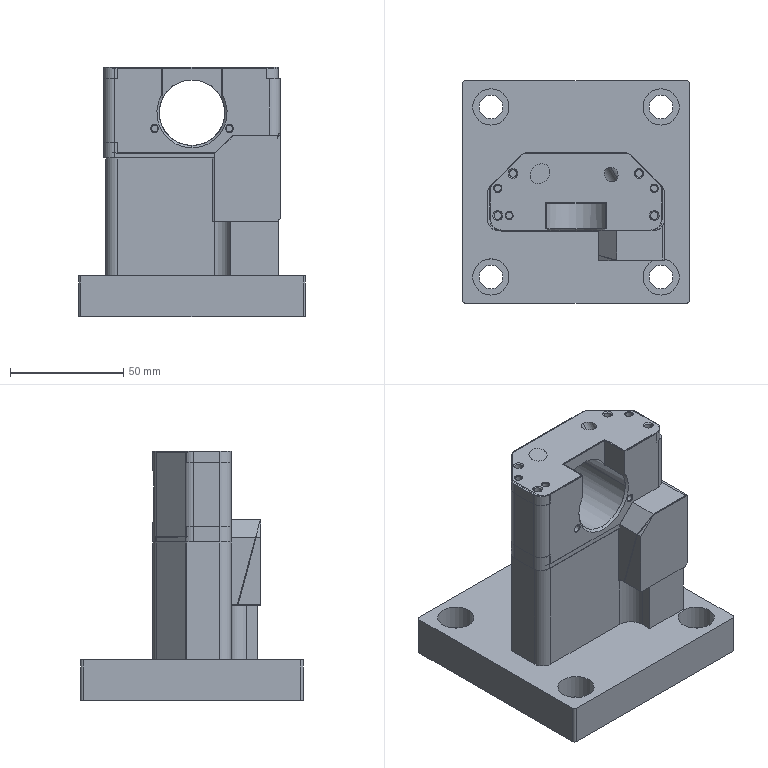NC program | NX | posted with a generic post | part box 100 x 98 x 110 mm
Lines 1 to 816 of 6635:
N10 G17 G21 G94 G90
(ADAPTIVE_MILLING_1 , TOOL : D16-48-D16-100-3T-ROUGH)
N12 T02 M6
N14 G54
N16 G17 G0 G90 X-56.885 Y-40.205 B0. C0. S6500 M3
N18 G43 Z71. H2
N20 Z43.15
N22 G94 G1 X-56.737 Y-40.182 Z42.213 F3000.
N24 X-56.588 Y-40.16 Z41.842
N26 X-56.44 Y-40.138 Z41.57
N28 X-56.291 Y-40.116 Z41.35
N30 X-56.143 Y-40.093 Z41.166
N32 X-55.995 Y-40.071 Z41.008
N34 X-55.846 Y-40.049 Z40.87
N36 X-55.698 Y-40.027 Z40.75
N38 X-55.55 Y-40.004 Z40.645
N40 X-55.401 Y-39.982 Z40.552
N42 X-55.253 Y-39.96 Z40.471
N44 X-55.105 Y-39.937 Z40.4
N46 X-54.956 Y-39.915 Z40.34
N48 X-54.808 Y-39.893 Z40.288
N50 X-54.66 Y-39.871 Z40.245
N52 X-54.511 Y-39.848 Z40.211
N54 X-54.363 Y-39.826 Z40.184
N56 X-54.215 Y-39.804 Z40.165
N58 X-54.066 Y-39.782 Z40.154
N60 X-53.918 Y-39.759 Z40.15
N62 X-51.733 Y-39.431
N64 G3 X-50.362 Y-37.706 R1.616
N66 G2 X-50.32 Y-34.589 R11.935
N68 G3 X-50.025 Y-25.185 R132.104
N70 G1 X-50. Y-12.98
N72 X-49.999 Y17.769
N74 G2 X-47.614 Y23.395 R8.513
N76 X-42.154 Y26.798 R13.179
N78 X-35.417 Y28.08 R28.008
N80 X-26.55 Y28.398 R123.992
N82 G1 X-12.675 Y28.431
N84 X39.401 Y28.429
N86 G2 X45.01 Y26.001 R8.56
N88 X48.428 Y20.406 R13.296
N90 X49.673 Y13.535 R29.032
N92 X49.978 Y3.542 R145.98
N94 G1 X50. Y-8.708
N96 X49.999 Y-30.87
N98 G2 X47.636 Y-36.505 R8.508
N100 X42.184 Y-39.92 R13.098
N102 X35.323 Y-41.215 R28.218
N104 X24.956 Y-41.538 R142.942
N106 G1 X12.831 Y-41.56
N108 X-38.711 Y-41.565
N110 G2 X-43.908 Y-39.391 R8.253
N112 X-47.391 Y-33.973 R12.678
N114 X-48.662 Y-27.362 R26.87
N116 X-48.98 Y-17.119 R138.758
N118 G1 X-49. Y-5.369
N120 X-48.995 Y14.156
N122 G2 X-44.813 Y22.643 R11.417
N124 X-38.379 Y25.922 R17.037
N126 X-30.735 Y27.117 R37.582
N128 X-19.116 Y27.415 R192.657
N130 G1 X-8.366 Y27.431
N132 X35.711 Y27.427
N134 G2 X44.199 Y23.258 R11.416
N136 X47.512 Y16.729 R17.072
N138 X48.682 Y9.208 R37.658
N140 X48.981 Y-2.036 R184.867
N142 G1 X48.999 Y-12.661
N144 X48.995 Y-27.28
N146 G2 X44.631 Y-35.925 R11.455
N148 X38.055 Y-39.14 R17.391
N150 X30.4 Y-40.267 R39.59
N152 X18.155 Y-40.547 R216.039
N154 G1 X8.905 Y-40.56
N156 X-34.711 Y-40.566
N158 G2 X-43.314 Y-36.39 R11.266
N160 X-46.587 Y-29.818 R17.057
N162 X-47.7 Y-22.413 R38.181
N164 X-47.987 Y-10.418 R203.457
N166 G1 X-47.999 Y-0.793
N168 G2 X-47.978 Y11.392 R882.053
N170 X-42.319 Y21.918 R13.288
N172 X-35.382 Y25.006 R19.979
N174 X-26.971 Y26.15 R45.911
N176 X-13.975 Y26.42 R250.02
N178 G1 X-4.35 Y26.43
N180 X32.086 Y26.429
N182 G2 X38.948 Y24.812 R13.899
N184 X44.742 Y18.723 R14.548
N186 X47.104 Y11.243 R24.627
N188 X47.861 Y2.156 R69.648
N190 X47.997 Y-13.218 R577.956
N192 X47.972 Y-24.654 R605.431
N194 X42.312 Y-35.05 R13.267
N196 X35.139 Y-38.192 R20.2
N198 X26.721 Y-39.291 R47.551
N200 X12.475 Y-39.553 R284.691
N202 G1 X4.225 Y-39.56
N204 X-31.335 Y-39.564
N206 G2 X-38.711 Y-37.564 R13.487
N208 X-44.102 Y-31.274 R14.868
N210 X-46.22 Y-23.842 R26.112
N212 X-46.894 Y-14.372 R79.249
N214 X-46.999 Y3.002 R851.623
N216 X-46.939 Y9.401 R131.04
N218 X-40.169 Y21.069 R14.609
N220 X-32.657 Y24.096 R22.601
N222 X-23.607 Y25.181 R54.343
N224 X-8.485 Y25.425 R334.897
N226 G1 X-1.61 Y25.43
N228 X28.915 Y25.429
N230 G2 X34.482 Y24.776 R19.528
N232 X42.634 Y18.602 R14.637
N234 X45.663 Y11.091 R22.586
N236 X46.742 Y2.166 R53.819
N238 X46.993 Y-13.081 R329.877
N240 X46.964 Y-22.08 R344.498
N242 X44.364 Y-30.176 R14.873
N244 X37.58 Y-35.614 R16.432
N246 X29.765 Y-37.748 R28.844
N248 X19.921 Y-38.444 R85.653
N250 X1.046 Y-38.56 R885.601
N252 G1 X-28.085 Y-38.564
N254 G2 X-33.65 Y-37.896 R19.153
N256 X-41.719 Y-31.705 R14.562
N258 X-44.704 Y-24.187 R22.662
N260 X-45.755 Y-15.259 R54.73
N262 X-45.992 Y-1.012 R322.025
N264 X-45.945 Y6.862 R209.476
N266 X-43.914 Y14.394 R16.668
N268 X-37.081 Y20.814 R16.454
N270 X-29.017 Y23.388 R27.307
N272 X-19.313 Y24.256 R73.092
N274 X-2.314 Y24.428 R541.419
N276 G1 X25.961 Y24.429
N278 G2 X31.558 Y23.989 R26.965
N280 X41.465 Y17.077 R15.491
N282 X44.553 Y9.453 R23.605
N284 X45.709 Y0.287 R54.619
N286 X45.989 Y-14.334 R295.948
N288 X45.906 Y-20.582 R95.145
N290 X42.831 Y-29.171 R15.836
N292 X35.625 Y-34.633 R17.635
N294 X27.542 Y-36.743 R31.272
N296 X17.446 Y-37.439 R91.485
N298 X-1.803 Y-37.56 R888.945
N300 G1 X-25.46 Y-37.562
N302 G2 X-31.169 Y-37.01 R23.929
N304 X-40.551 Y-30.162 R15.425
N306 X-43.62 Y-22.412 R23.796
N308 X-44.734 Y-13.114 R56.809
N310 X-44.951 Y4.382 R306.489
N312 X-43.611 Y11.214 R19.554
N314 X-36.477 Y19.2 R16.579
N316 X-28.528 Y22.101 R26.152
N318 X-18.847 Y23.178 R63.148
N320 X-2.725 Y23.424 R380.785
N322 G1 X4.15 Y23.429
N324 X23.8 Y23.427
N326 G2 X29.771 Y22.955 R29.934
N328 X40.427 Y15.466 R16.289
N330 X43.558 Y7.471 R25.044
N332 X44.72 Y-2.198 R59.034
N334 X44.947 Y-17.444 R256.134
N336 X43.633 Y-24.281 R19.663
N338 X36.608 Y-32.247 R16.569
N340 X28.551 Y-35.222 R25.928
N342 X18.746 Y-36.31 R63.537
N344 X2.624 Y-36.554 R385.545
N346 G1 X-4.251 Y-36.56
N348 X-22.96 Y-36.561
N350 G2 X-28.93 Y-36.077 R29.329
N352 X-39.456 Y-28.627 R16.21
N354 X-42.552 Y-20.738 R24.98
N356 X-43.714 Y-11.194 R58.416
N358 X-43.921 Y2.676 R191.786
N360 X-42.612 Y9.519 R20.813
N362 X-35.365 Y17.907 R17.11
N364 X-27.077 Y21.017 R26.557
N366 X-17.027 Y22.162 R64.138
N368 X-1.406 Y22.421 R359.586
N370 G1 X6.844 Y22.428
N372 X21.336 Y22.427
N374 G2 X27.565 Y22.023 R36.993
N376 X39.255 Y14.153 R16.957
N378 X42.44 Y6.164 R25.668
N380 X43.675 Y-3.497 R58.226
N382 X43.904 Y-15.867 R156.374
N384 X42.486 Y-22.938 R20.39
N386 X35.181 Y-31.143 R17.173
N388 X26.868 Y-34.186 R27.044
N390 X16.815 Y-35.3 R65.737
N392 X0.318 Y-35.554 R391.668
N394 G1 X-6.557 Y-35.559
N396 X-20.085 Y-35.561
N398 G2 X-26.319 Y-35.213 R40.275
N400 X-38.402 Y-27.115 R16.941
N402 X-41.53 Y-18.984 R26.096
N404 X-42.713 Y-9.066 R61.493
N406 X-42.876 Y1.055 R124.215
N408 X-41.416 Y8.372 R21.436
N410 X-34.005 Y16.803 R17.662
N412 X-25.863 Y19.901 R27.04
N414 X-15.948 Y21.114 R62.015
N416 X-0.077 Y21.418 R322.023
N418 G1 X9.548 Y21.427
N420 G2 X21.697 Y21.388 R659.225
N422 X28.477 Y20.39 R25.036
N424 X38.259 Y12.625 R17.561
N426 X41.476 Y4.261 R26.907
N428 X42.691 Y-5.78 R62.743
N430 X42.826 Y-14.65 R92.117
N432 X41.063 Y-22.274 R20.204
N434 X33.684 Y-30.116 R17.819
N436 X25.377 Y-33.131 R27.885
N438 X15.326 Y-34.275 R66.109
N440 X-0.42 Y-34.55 R353.217
N442 G1 X-8.67 Y-34.559
N444 G2 X-20.835 Y-34.52 R627.473
N446 X-27.492 Y-33.541 R24.81
N448 X-37.297 Y-25.753 R17.501
N450 X-40.496 Y-17.386 R26.951
N452 X-41.703 Y-7.219 R63.63
N454 X-41.73 Y0.776 R63.896
N456 X-39.361 Y8.998 R19.551
N458 X-31.841 Y16.186 R18.657
N460 X-23.353 Y19.073 R29.671
N462 X-12.92 Y20.17 R72.683
N464 X4.327 Y20.422 R423.71
N466 G1 X11.202 Y20.427
N468 G2 X20.585 Y20.356 R267.632
N470 X27.702 Y19.122 R24.347
N472 X37.307 Y11.071 R18.155
N474 X40.485 Y2.552 R28.12
N476 X41.708 Y-8.117 R66.144
N478 X41.556 Y-15.231 R42.135
N480 X32.931 Y-28.678 R17.947
N482 X24.577 Y-31.94 R27.303
N484 X14.667 Y-33.207 R61.606
N486 X-0.578 Y-33.544 R290.453
N488 G1 X-11.578 Y-33.559
N490 G2 X-20.209 Y-33.463 R178.586
N492 X-27.523 Y-31.969 R22.618
N494 X-36.369 Y-24.155 R18.163
N496 X-39.489 Y-15.738 R28.141
N498 X-40.666 Y-1.194 R61.873
N500 X-38.682 Y6.89 R20.653
N502 X-30.912 Y14.894 R18.781
N504 X-22.467 Y17.924 R29.31
N506 X-11.921 Y19.13 R69.186
N508 X4.325 Y19.417 R361.409
N510 X18.2 Y19.377 R613.553
N512 X25.241 Y18.419 R28.599
N514 X36.144 Y9.914 R18.54
N516 X39.381 Y1.424 R28.401
N518 X40.594 Y-11.988 R55.222
N520 X38.515 Y-20.291 R20.184
N522 X30.766 Y-28.096 R18.808
N524 X22.189 Y-31.105 R29.746
N526 X11.763 Y-32.266 R70.65
N528 X-5.234 Y-32.551 R382.948
N530 X-17.483 Y-32.504 R470.412
N532 X-24.396 Y-31.527 R27.9
N534 X-35.1 Y-23.172 R18.455
N536 X-38.338 Y-14.811 R27.977
N538 X-39.5 Y-2.275 R48.395
N540 X-37.123 Y6.453 R20.027
N542 X-29.457 Y13.912 R19.217
N544 X-20.637 Y16.977 R30.448
N546 X-9.835 Y18.145 R73.801
N548 X7.662 Y18.42 R411.362
N550 X17.535 Y18.332 R229.778
N552 X24.782 Y17.099 R26.546
N554 X35.03 Y8.718 R18.923
N556 X38.384 Y-0.143 R29.074
N558 X39.392 Y-11.067 R43.089
N560 X36.714 Y-20.213 R19.386
N562 X28.974 Y-27.287 R19.454
N564 X20.203 Y-30.184 R31.503
N566 X9.393 Y-31.294 R77.133
N568 X-7.729 Y-31.552 R429.437
N570 X-16.602 Y-31.465 R200.678
N572 X-23.848 Y-30.23 R26.387
N574 X-34.069 Y-21.832 R18.881
N576 X-37.371 Y-13.1 R28.888
N578 X-38.256 Y-2.92 R37.59
N580 X-34.78 Y7.115 R19.055
N582 X-26.856 Y13.521 R20.464
N584 X-17.776 Y16.217 R34.328
N586 X-6.452 Y17.215 R89.134
N588 X14.92 Y17.367 R468.732
N590 X22.219 Y16.435 R31.978
N592 X33.937 Y7.516 R19.297
N594 X37.361 Y-1.577 R29.292
N596 X38.091 Y-10.767 R32.807
N598 X29.508 Y-25.154 R18.422
N600 X20.969 Y-28.686 R27.691
N602 X10.583 Y-30.136 R60.771
N604 X-4.535 Y-30.534 R261.029
N606 X-15.034 Y-30.457 R229.195
N608 X-22.409 Y-29.229 R27.63
N610 X-33.052 Y-20.497 R19.274
N612 X-36.486 Y-10.886 R29.362
N614 X-36.799 Y-2.179 R27.378
N616 X-28.604 Y10.743 R18.461
N618 X-20.027 Y14.431 R27.428
N620 X-9.778 Y15.952 R58.414
N622 X4.088 Y16.388 R225.599
N624 X14.461 Y16.315 R208.549
N626 X21.964 Y15.091 R28.827
N628 X32.87 Y6.301 R19.628
N630 X36.627 Y-5.021 R29.285
N632 X36.056 Y-13.816 R21.747
N634 X28.557 Y-23.866 R18.306
N636 X19.97 Y-27.564 R27.369
N638 X9.721 Y-29.083 R58.654
N640 X-5.395 Y-29.528 R242.488
N642 X-14.517 Y-29.388 R129.556
N644 X-22.198 Y-27.8 R25.596
N646 X-31.983 Y-19.279 R19.641
N648 X-35.62 Y-5.029 R27.098
N650 X-27.736 Y9.396 R18.221
N652 X-19.469 Y13.192 R26.585
N654 X-9.247 Y14.871 R54.684
N656 X5.241 Y15.381 R206.257
N658 X14.362 Y15.218 R113.494
N660 X22.148 Y13.529 R25.672
N662 X31.918 Y4.911 R19.991
N664 X35.4 Y-8.094 R25.444
N666 X27.944 Y-22.318 R17.842
N668 X19.493 Y-26.297 R26.146
N670 X9.399 Y-27.984 R53.896
N672 X-4.963 Y-28.509 R200.139
N674 X-13.708 Y-28.326 R99.733
N676 X-21.592 Y-26.492 R24.816
N678 X-31.116 Y-17.723 R19.984
N680 X-34.164 Y-5.853 R23.484
N682 X-27.199 Y7.764 R17.675
N684 X-18.927 Y11.928 R25.352
N686 X-9.107 Y13.746 R50.121
N688 X5.126 Y14.358 R171.985
N690 X13.744 Y14.135 R85.535
N692 X21.938 Y12.044 R24.427
N694 X31.299 Y2.906 R20.376
N696 X33.883 Y-7.671 R21.757
N698 X27.536 Y-20.534 R17.229
N700 X19.275 Y-24.924 R24.472
N702 X9.353 Y-26.845 R48.428
N704 X-4.504 Y-27.48 R161.733
N706 X-13.12 Y-27.231 R78.292
N708 X-21.395 Y-24.972 R23.686
N710 X-30.848 Y-14.861 R20.337
N712 X-32.463 Y-4.616 R19.331
N714 X-26.283 Y6.366 R17.162
N716 X-18.15 Y10.718 R24.431
N718 X-8.356 Y12.668 R47.689
N720 X10.372 Y13.252 R148.984
N722 X18.127 Y12.014 R30.686
N724 X32.213 Y-5.312 R20.183
N726 X26.806 Y-18.907 R16.489
N728 X18.883 Y-23.56 R23.107
N730 X9.386 Y-25.672 R43.694
N732 X-4.461 Y-26.442 R132.029
N734 X-12.822 Y-26.083 R60.203
N736 X-21.752 Y-23.06 R22.292
N738 X-30.735 Y-9.76 R19.35
N740 X-26.025 Y4.269 R16.135
N742 X-18.119 Y9.214 R22.417
N744 X-8.775 Y11.44 R41.528
N746 X9.565 Y12.189 R116.003
N748 X17.42 Y10.809 R29.248
N750 X29.52 Y-0.727 R19.418
N752 X26.199 Y-17.008 R15.583
N754 X18.558 Y-22.115 R21.467
N756 X9.256 Y-24.489 R39.196
N758 X-4.831 Y-25.39 R108.385
N760 X-12.926 Y-24.835 R45.533
N762 X-22.552 Y-20.614 R20.979
N764 X-28.744 Y-10.981 R17.552
N766 X-25.355 Y2.321 R15.122
N768 X-17.975 Y7.658 R20.555
N770 X-8.847 Y10.21 R36.601
N772 X8.728 Y11.112 R92.536
N774 X16.917 Y9.517 R27.854
N776 X26.436 Y1.819 R18.73
N778 X25.351 Y-15.128 R14.581
N780 X18.133 Y-20.63 R19.791
N782 X9.532 Y-23.203 R34.399
N784 X-4.284 Y-24.311 R85.783
N786 X-12.491 Y-23.634 R39.783
N788 X-21.782 Y-19.202 R20.242
N790 X-26.884 Y-10.793 R15.424
N792 X-24.071 Y0.859 R14.209
N794 X-16.905 Y6.435 R19.497
N796 X-8.072 Y9.086 R34.247
N798 X7.995 Y10.011 R74.707
N800 X16.274 Y8.255 R26.491
N802 X24.04 Y2.318 R17.591
N804 X24.294 Y-13.173 R13.493
N806 X17.705 Y-19.032 R18.06
N808 X9.342 Y-21.94 R30.46
N810 X-7.325 Y-23.097 R67.662
N812 X-15.467 Y-21.303 R25.558
N814 X-22.541 Y-15.899 R16.613
N816 X-23.18 Y-1.523 R12.975
N818 X-16.814 Y4.611 R17.312
N820 X-8.397 Y7.715 R29.048
N822 X7.388 Y8.877 R59.899
N824 X15.627 Y6.964 R24.802
N826 X22.062 Y1.935 R15.623
N828 X22.92 Y-11.206 R12.412
N830 X16.932 Y-17.464 R16.395
N832 X8.812 Y-20.694 R27.127
N834 X-6.835 Y-21.94 R54.242
N836 X-14.807 Y-19.989 R23.437
N838 X-20.733 Y-15.113 R14.174
N840 X-21.437 Y-3.087 R11.966
N842 X-15.55 Y3.276 R15.99
N844 X-7.591 Y6.512 R26.353
N846 X7.179 Y7.676 R47.817
N848 X14.763 Y5.715 R22.244
N850 X20.403 Y0.735 R12.949
N852 X20.865 Y-9.951 R11.505
N854 X15.319 Y-16.264 R15.291
N856 X7.523 Y-19.575 R25.019
N858 X-6.616 Y-20.717 R43.089
N860 X-13.591 Y-18.856 R20.486
N862 X-19.066 Y-13.559 R11.694
N864 X-19.035 Y-3.884 R11.205
N866 X-13.507 Y2.293 R15.092
N868 X-5.798 Y5.496 R24.694
N870 X6.984 Y6.417 R37.765
N872 X13.441 Y4.573 R18.418
N874 X19.141 Y-3.484 R10.505
N876 X16.905 Y-11.621 R11.616
N878 X10.678 Y-16.716 R16.592
N880 X1.833 Y-19.288 R28.96
N882 X-7.381 Y-19.276 R30.623
N884 X-12.847 Y-17.238 R14.001
N886 X-16.944 Y-6.618 R9.897
N888 X-12.787 Y0.066 R12.881
N890 X-5.683 Y3.922 R19.713
N892 X6.667 Y5.083 R29.045
N894 X11.824 Y3.303 R12.563
N896 X15.928 Y-6.115 R9.363
N898 X12.061 Y-13.089 R12.147
N900 X5.016 Y-17.036 R18.525
N902 X-5.477 Y-18.093 R24.979
N904 X-10.71 Y-15.913 R9.896
N906 X-13.65 Y-7.689 R8.937
N908 X-9.995 Y-0.995 R11.714
N910 X-2.938 Y2.916 R17.429
N912 X4.721 Y3.748 R20.39
N914 X12.159 Y-4.269 R8.111
N916 X9.554 Y-11.257 R10.475
N918 X2.679 Y-15.715 R15.051
N920 X-2.23 Y-16.538 R14.881
N922 X-8.827 Y-11.184 R7.024
N924 X-7.719 Y-4.212 R9.092
N926 X-1.402 Y0.889 R12.075
N928 X2.442 Y0.365 R4.734
N930 X6.261 Y-5.107 R8.144
N932 G1 X6.388 Y-5.846
N934 X6.409 Y-5.994 Z40.154
N936 X6.43 Y-6.143 Z40.165
N938 X6.451 Y-6.291 Z40.184
N940 X6.472 Y-6.44 Z40.211
N942 X6.492 Y-6.588 Z40.245
N944 X6.513 Y-6.737 Z40.288
N946 X6.534 Y-6.886 Z40.34
N948 X6.555 Y-7.034 Z40.4
N950 X6.576 Y-7.183 Z40.471
N952 X6.596 Y-7.331 Z40.552
N954 X6.617 Y-7.48 Z40.645
N956 X6.638 Y-7.628 Z40.75
N958 X6.659 Y-7.777 Z40.87
N960 X6.68 Y-7.925 Z41.008
N962 X6.701 Y-8.074 Z41.166
N964 X6.721 Y-8.222 Z41.35
N966 X6.742 Y-8.371 Z41.57
N968 X6.763 Y-8.52 Z41.842
N970 X6.784 Y-8.668 Z42.213
N972 X6.805 Y-8.817 Z43.15
N974 G0 Z71.
(ADAPTIVE_MILLING_1_COPY , TOOL : D16-48-D16-100-3T-ROUGH)
N976 X-58.104 Y-13.402
N978 Z3.
N980 G1 X-57.954 Y-13.401 Z2.063
N982 X-57.804 Y-13.399 Z1.692
N984 X-57.654 Y-13.398 Z1.42
N986 X-57.504 Y-13.396 Z1.2
N988 X-57.354 Y-13.395 Z1.016
N990 X-57.204 Y-13.393 Z0.858
N992 X-57.054 Y-13.391 Z0.72
N994 X-56.904 Y-13.39 Z0.6
N996 X-56.754 Y-13.388 Z0.495
N998 X-56.604 Y-13.387 Z0.402
N1000 X-56.454 Y-13.385 Z0.321
N1002 X-56.304 Y-13.384 Z0.25
N1004 X-56.154 Y-13.382 Z0.19
N1006 X-56.004 Y-13.38 Z0.138
N1008 X-55.854 Y-13.379 Z0.095
N1010 X-55.704 Y-13.377 Z0.061
N1012 X-55.554 Y-13.376 Z0.034
N1014 X-55.404 Y-13.374 Z0.015
N1016 X-55.254 Y-13.373 Z0.004
N1018 X-55.104 Y-13.371 Z0.
N1020 X-52.595 Y-13.345
N1022 G3 X-51.099 Y-12.298 R1.616
N1024 X-50.374 Y-8.84 R12.888
N1026 X-50.039 Y-0.285 R101.881
N1028 G1 X-50.001 Y11.645
N1030 G2 X-49.977 Y18.269 R246.209
N1032 X-47.177 Y23.842 R8.816
N1034 X-41.44 Y27.029 R13.966
N1036 X-34.42 Y28.156 R32.117
N1038 X-23.55 Y28.418 R184.549
N1040 G1 X-12.05 Y28.431
N1042 X39.301
N1044 G2 X44.844 Y26.153 R8.484
N1046 X48.314 Y20.737 R12.964
N1048 X49.634 Y14.009 R27.356
N1050 X49.969 Y4.642 R123.746
N1052 G1 X49.999 Y-8.733
N1054 Y-30.883
N1056 G2 X47.627 Y-36.514 R8.513
N1058 X42.172 Y-39.925 R13.111
N1060 X35.56 Y-41.195 R27.691
N1062 X25.693 Y-41.53 R130.266
N1064 G1 X11.818 Y-41.56
N1066 X-39.335 Y-41.567
N1068 G2 X-44.962 Y-39.183 R8.512
N1070 X-48.365 Y-33.723 R13.157
N1072 X-49.648 Y-26.987 R27.985
N1074 X-49.942 Y-15.62 R121.457
N1076 X-49.408 Y-8.984 R438.125
N1078 G3 X-49.027 Y4.188 R208.616
N1080 G2 X-48.981 Y14.52 R952.673
N1082 X-44.634 Y22.793 R11.49
N1084 X-38.057 Y26.011 R17.399
N1086 X-30.277 Y27.148 R39.746
N1088 X-18.782 Y27.413 R208.726
N1090 G1 X-6.032 Y27.431
N1092 X35.711 Y27.426
N1094 G2 X44.199 Y23.258 R11.415
N1096 X47.513 Y16.73 R17.067
N1098 X48.691 Y9.084 R37.977
N1100 X48.98 Y-2.536 R194.558
N1102 G1 X48.997 Y-11.286
N1104 X48.999 Y-27.03
N1106 G2 X44.632 Y-35.926 R11.452
N1108 X38.054 Y-39.14 R17.391
N1110 X30.274 Y-40.273 R39.898
N1112 X17.779 Y-40.544 R228.031
N1114 G1 X6.654 Y-40.56
N1116 X-35.71 Y-40.562
N1118 G2 X-44.198 Y-36.395 R11.411
N1120 X-47.512 Y-29.865 R17.072
N1122 X-48.682 Y-22.344 R37.742
N1124 X-48.638 Y-12.853 R65.901
N1126 G3 X-48.023 Y7.18 R301.717
N1128 G2 X-47.948 Y12.034 R86.033
N1130 X-42.317 Y21.922 R13.278
N1132 X-35.38 Y25.007 R19.986
N1134 X-26.845 Y26.157 R46.187
N1136 X-13.349 Y26.418 R272.072
N1138 G1 X-1.849 Y26.43
N1140 X32.111 Y26.429
N1142 G2 X39.076 Y24.741 R13.86
N1144 X44.742 Y18.724 R14.574
N1146 X47.105 Y11.242 R24.618
N1148 X47.859 Y2.155 R69.679
N1150 X47.998 Y-15.094 R696.648
N1152 X47.977 Y-24.743 R485.289
N1154 X46.233 Y-30.817 R13.579
N1156 G3 X45.884 Y-32.388 R15.193
N1158 G2 X44.218 Y-35.486 R8.882
N1160 X40.95 Y-37.913 R9.926
N1162 X37.897 Y-38.577 R8.772
N1164 X20.207 Y-39.509 R172.523
N1166 X7.082 Y-39.558 R864.385
N1168 G1 X-31.836 Y-39.565
N1170 G2 X-38.052 Y-38.394 R14.528
N1172 X-44.376 Y-32.517 R14.089
N1174 X-46.949 Y-25.242 R22.937
N1176 X-47.637 Y-15.783 R46.19
N1178 X-47.239 Y-4.883 R909.042
N1180 G3 X-47.2 Y-0.722 R100.176
N1182 X-47.005 Y8.71 R694.056
N1184 G2 X-44.922 Y16.214 R15.361
N1186 X-38.312 Y22.144 R15.862
N1188 X-30.565 Y24.5 R26.855
N1190 X-23.487 Y25.191 R67.463
N1192 G1 X-22.751 Y25.337
N1194 X-21.028 Y25.45
N1196 X22.114 Y25.445
N1198 G2 X30.593 Y25.393 R336.528
N1200 X38.991 Y22.525 R14.793
N1202 X44.182 Y15.726 R16.692
N1204 X46.265 Y7.643 R30.031
N1206 X46.72 Y2.79 R102.116
N1208 G1 X47.087 Y1.001
N1210 X47.2 Y-0.722
N1212 Y-12.299
N1214 G3 X47.002 Y-21.573 R222.409
N1216 G2 X46.225 Y-26.753 R22.013
N1218 G1 X46.2 Y-26.942
N1220 Y-30.054
N1222 G2 X45.479 Y-33.497 R8.883
N1224 X42.944 Y-36.692 R8.748
N1226 X39.862 Y-38.295 R8.922
N1228 X37.581 Y-38.587 R9.484
N1230 G1 X17.727 Y-38.581
N1232 X8.788 Y-38.559
N1234 X-28.961 Y-38.564
N1236 G2 X-34.526 Y-37.899 R19.358
N1238 X-42.635 Y-31.738 R14.639
N1240 X-45.723 Y-23.855 R22.343
N1242 X-46.456 Y-16.651 R43.504
N1244 G3 X-46.836 Y-15.327 R24.923
N1246 G2 X-47.2 Y-12.273 R15.354
N1248 G1 Y-3.523
N1250 G3 X-49.939 Y-2.4 R1.6
N1252 X-50.356 Y-3.121 Z0.027 R1.79
N1254 G1 X-51.152 Y-5.304 Z0.1
N1256 X-52.138 Y-8.011 F15000.
N1258 G3 X-52.235 Y-8.558 R1.671
N1260 G1 X-52.237 Y-10.974
N1262 X-52.225 Y-13.39
N1264 G3 X-51.459 Y-20.349 R39.984
N1266 G1 X-50.868 Y-23.254
N1268 G3 X-48.91 Y-29.873 R49.325
N1270 G1 X-48.468 Y-31.063
N1272 X-48.012 Y-32.249
N1274 G3 X-45.751 Y-36.119 R16.03
N1276 X-43.777 Y-38.106 R13.541
N1278 X-41.971 Y-39.527 R34.655
N1280 X-36.881 Y-42.176 R20.204
N1282 X-32.28 Y-43.055 R16.86
N1284 X-20.432 Y-43.426 R247.094
N1286 G1 X13.234 Y-43.621
N1288 G3 X13.8 Y-43.522 R1.662
N1290 G1 X16.685 Y-42.451
N1292 X17.764 Y-42.055 Z0.064 F3000.
N1294 X18.839 Y-41.646 Z0.027
N1296 G3 X19.502 Y-41.108 Z0. R1.602
N1298 X18.269 Y-38.586 R1.6
N1300 G2 X15.465 Y-38.188 R12.379
N1302 G3 X9.552 Y-37.686 R41.198
N1304 X-6.962 Y-37.562 R604.321
N1306 G1 X-26.362 Y-37.563
N1308 G2 X-31.95 Y-37.039 R24.423
N1310 X-41.467 Y-30.21 R15.472
N1312 X-44.582 Y-22.072 R22.776
N1314 G1 X-45.002 Y-19.633
N1316 X-45.102 Y-19.371
N1318 G2 X-46.499 Y-16.442 R12.643
N1320 G3 X-49.165 Y-15.777 R1.6
N1322 X-49.637 Y-16.896 Z0.039 R1.692
N1324 G1 X-49.825 Y-18.808 Z0.1
N1326 X-50.134 Y-21.946 F15000.
N1328 G3 X-50.059 Y-22.608 R1.626
N1330 G1 X-49.459 Y-24.418
N1332 X-48.844 Y-26.222
N1334 G3 X-43.507 Y-35.772 R33.376
N1336 X-34.771 Y-41.386 R16.497
N1338 X-32.794 Y-41.783 R21.354
N1340 X-27.754 Y-42.256 R38.075
N1342 G1 X10.752 Y-43.288
N1344 G3 X11.412 Y-43.165 R1.625
N1346 G1 X14.296 Y-41.96
N1348 X15.173 Y-41.597 Z0.07 F3000.
N1350 X16.044 Y-41.223 Z0.04
N1352 G3 X16.858 Y-40.296 Z0. R1.599
N1354 X15.787 Y-38.254 R1.6
N1356 X12.309 Y-37.331 R65.438
N1358 X5.641 Y-36.721 R43.905
N1360 X-10.838 Y-36.563 R507.212
N1362 G1 X-23.112 Y-36.564
N1364 G2 X-28.848 Y-36.257 R37.738
N1366 X-40.573 Y-28.332 R16.239
N1368 X-42.951 Y-22.727 R25.365
N1370 G3 X-43.473 Y-21.426 R4.994
N1372 G2 X-45.127 Y-19.328 R13.176
N1374 G3 X-47.954 Y-19.443 R1.6
N1376 X-48.055 Y-20.578 Z0.037 R1.707
N1378 G1 X-47.688 Y-22.546 Z0.1
N1380 X-47.065 Y-25.887 F15000.
N1382 X-47.024 Y-26.048
N1384 X-46.97 Y-26.206
N1386 X-46.487 Y-27.38
N1388 X-45.989 Y-28.549
N1390 G3 X-44.26 Y-31.436 R15.357
N1392 G1 X-43.366 Y-32.612
N1394 X-42.465 Y-33.782
N1396 G3 X-40.208 Y-36.397 R39.718
N1398 X-36.999 Y-38.747 R12.444
N1400 X-33.86 Y-39.959 R15.349
N1402 X-30.749 Y-40.687 R36.352
N1404 X-27.086 Y-41.086 R27.217
N1406 G1 X7.868 Y-42.495
N1408 G3 X8.546 Y-42.374 R1.623
N1410 G1 X11.421 Y-41.18
N1412 X12.306 Y-40.816 Z0.07 F3000.
N1414 X13.187 Y-40.441 Z0.039
N1416 G3 X13.998 Y-39.533 Z0. R1.599
N1418 X12.903 Y-37.46 R1.6
N1420 X8.797 Y-36.387 R98.415
N1422 X2.47 Y-35.757 R43.754
N1424 X-11.842 Y-35.566 R367.925
N1426 G2 X-23.737 Y-35.524 R596.69
N1428 X-30.492 Y-34.404 R22.346
N1430 X-39.323 Y-27.105 R16.856
N1432 X-41.331 Y-23.408 R81.229
N1434 G3 X-41.652 Y-23.019 R8.516
N1436 G2 X-43.618 Y-21.258 R11.986
N1438 G3 X-46. Y-21.329 R1.6
N1440 X-46.36 Y-22.595 Z0.043 R1.616
N1442 G1 X-46.096 Y-24.384 Z0.1
N1444 X-45.613 Y-27.654 F15000.
N1446 G3 X-45.461 Y-28.136 R1.707
N1448 G1 X-45.168 Y-28.725
N1450 X-44.864 Y-29.308
N1452 G3 X-43.849 Y-30.574 R5.409
N1454 G1 X-41.789 Y-32.473
N1456 X-39.719 Y-34.36
N1458 G3 X-35.988 Y-37.046 R23.959
N1460 X-33.623 Y-38.186 R19.254
N1462 X-31.482 Y-38.997 R33.504
N1464 X-27.01 Y-39.903 R19.94
N1466 X-15.179 Y-40.707 R257.471
N1468 G1 X4.367 Y-41.554
N1470 G3 X5.05 Y-41.433 R1.622
N1472 G1 X7.935 Y-40.234
N1474 X8.814 Y-39.873 Z0.07 F3000.
N1476 X9.688 Y-39.499 Z0.04
N1478 G3 X10.502 Y-38.577 Z0. R1.599
N1480 X9.402 Y-36.519 R1.6
N1482 G2 X7.144 Y-35.817 R13.948
N1484 G3 X2.042 Y-34.954 R24.022
N1486 X-8.518 Y-34.596 R150.735
N1488 G1 X-20.841 Y-34.546
N1490 G2 X-27.412 Y-33.826 R29.041
N1492 X-36.914 Y-27.678 R17.49
N1494 X-39.356 Y-24.467 R360.826
N1496 G3 X-40.124 Y-23.943 R2.316
N1498 G1 X-41.712 Y-22.973
N1500 G3 X-44.164 Y-23.618 R1.6
N1502 X-44.151 Y-24.892 Z0.041 R1.617
N1504 G1 X-43.394 Y-26.585 Z0.1
N1506 X-42.042 Y-29.614 F15000.
N1508 G3 X-41.712 Y-30.093 R1.659
N1510 G1 X-38.915 Y-32.89
N1512 G3 X-32.347 Y-37.14 R18.59
N1514 X-30.033 Y-37.964 R36.652
N1516 X-25.712 Y-38.852 R23.244
N1518 X-16.86 Y-39.635 R188.127
N1520 G1 X2.109 Y-40.852
N1522 G3 X2.86 Y-40.719 R1.615
N1524 G1 X5.635 Y-39.49
N1526 X7.315 Y-38.741 Z0.042 F3000.
N1528 G3 X8.13 Y-37.746 Z0. R1.6
N1530 X7.144 Y-35.817 R1.6
N1532 G2 X6.203 Y-35.346 R9.652
N1534 G3 X2.08 Y-34.271 R15.479
N1536 X-6.757 Y-33.675 R77.13
N1538 X-18.861 Y-33.55 R843.056
N1540 G2 X-25.321 Y-32.931 R33.078
N1542 X-34.568 Y-27.917 R18.868
N1544 G3 X-37.357 Y-25.154 R229.539
N1546 X-37.843 Y-24.875 R3.608
N1548 G2 X-39.815 Y-24.106 R7.529
N1550 G3 X-41.884 Y-24.626 R1.6
N1552 X-42.08 Y-26.018 Z0.046 R1.612
N1554 G1 X-41.55 Y-27.643 Z0.1
N1556 X-41.022 Y-29.263 F15000.
N1558 G3 X-39.815 Y-30.336 R1.601
N1560 G1 X0.807 Y-38.461
N1562 X0.988 Y-38.485
N1564 X1.17 Y-38.492
N1566 X3.61 Y-38.417
N1568 X5.594 Y-38.352 Z0.037 F3000.
N1570 G3 X6.629 Y-37.847 Z0. R1.6
N1572 X6.203 Y-35.346 R1.6
N1574 G2 X5.527 Y-34.914 R4.764
N1576 G3 X2.226 Y-33.698 R11.034
N1578 X-4.751 Y-32.857 R43.852
N1580 X-16.909 Y-32.566 R291.619
N1582 G2 X-23.621 Y-31.956 R36.916
N1584 X-32.475 Y-27.782 R21.192
N1586 G3 X-35.396 Y-25.525 R77.736
N1588 X-36.534 Y-25.205 R2.782
N1590 G2 X-37.963 Y-24.839 R32.308
N1592 G3 X-40. Y-26.124 R1.6
N1594 X-39.659 Y-27.384 Z0.042 R1.617
N1596 G1 X-38.509 Y-28.794 Z0.1
N1598 X-37.282 Y-30.299 F15000.
N1600 G3 X-36.351 Y-30.857 R1.603
N1602 G1 X0.132 Y-38.03
N1604 X0.332 Y-38.054
N1606 X0.533 Y-38.057
N1608 X2.911 Y-37.919
N1610 X4.778 Y-37.806 Z0.041 F3000.
N1612 G3 X5.873 Y-37.186 Z0. R1.6
N1614 X5.527 Y-34.914 R1.6
N1616 X3.766 Y-33.77 R11.305
N1618 X-1.012 Y-32.441 R17.909
N1620 X-9.941 Y-31.73 R74.721
N1622 G2 X-17.983 Y-31.479 R295.921
N1624 X-26.145 Y-29.756 R25.726